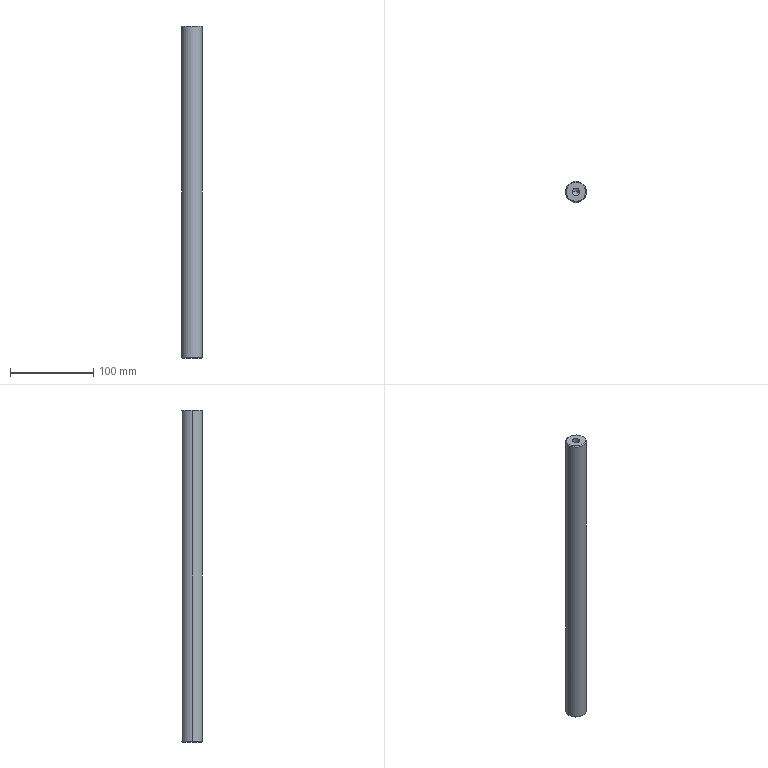Part | SolidWorks | features Chamfer 1, Extrusion 1, HoleWzd 1 | 1 solid | 12 faces | box 25 x 25 x 400 mm | volume 194835 mm3 | cone 6 | cylinder 4 | plane 2 | commonest cylinder face diameters 8.5 x2 25 x2
STEP:
#1=CARTESIAN_POINT('',(-4.25,0.,175.5));
#2=VERTEX_POINT('',#1);
#3=CARTESIAN_POINT('',(4.25,0.,175.5));
#4=VERTEX_POINT('',#3);
#5=CARTESIAN_POINT('',(0.,0.,175.5));
#6=DIRECTION('',(0.,0.,1.));
#7=DIRECTION('',(1.,0.,0.));
#8=AXIS2_PLACEMENT_3D('',#5,#6,#7);
#9=CIRCLE('',#8,4.25);
#10=EDGE_CURVE('',#2,#4,#9,.T.);
#11=ORIENTED_EDGE('',*,*,#10,.F.);
#12=CARTESIAN_POINT('',(-4.25,0.,200.));
#13=VERTEX_POINT('',#12);
#14=CARTESIAN_POINT('',(-4.25,0.,200.));
#15=DIRECTION('',(0.,0.,1.));
#16=VECTOR('',#15,1000.);
#17=LINE('',#14,#16);
#18=EDGE_CURVE('',#2,#13,#17,.T.);
#19=ORIENTED_EDGE('',*,*,#18,.T.);
#20=CARTESIAN_POINT('',(4.25,0.,200.));
#21=VERTEX_POINT('',#20);
#22=CARTESIAN_POINT('',(0.,0.,200.));
#23=DIRECTION('',(0.,0.,1.));
#24=DIRECTION('',(1.,0.,0.));
#25=AXIS2_PLACEMENT_3D('',#22,#23,#24);
#26=CIRCLE('',#25,4.25);
#27=EDGE_CURVE('',#13,#21,#26,.T.);
#28=ORIENTED_EDGE('',*,*,#27,.T.);
#29=CARTESIAN_POINT('',(4.25,0.,200.));
#30=DIRECTION('',(0.,0.,1.));
#31=VECTOR('',#30,1000.);
#32=LINE('',#29,#31);
#33=EDGE_CURVE('',#4,#21,#32,.T.);
#34=ORIENTED_EDGE('',*,*,#33,.F.);
#35=EDGE_LOOP('',(#11,#19,#28,#34));
#36=FACE_OUTER_BOUND('',#35,.T.);
#37=CARTESIAN_POINT('',(0.,0.,200.));
#38=DIRECTION('',(0.,0.,1.));
#39=DIRECTION('',(1.,0.,0.));
#40=AXIS2_PLACEMENT_3D('',#37,#38,#39);
#41=CYLINDRICAL_SURFACE('',#40,4.25);
#42=ADVANCED_FACE('',(#36),#41,.F.);
#43=CARTESIAN_POINT('',(0.,0.,172.946));
#44=VERTEX_POINT('',#43);
#45=CARTESIAN_POINT('',(4.25,0.,175.5));
#46=DIRECTION('',(0.8572,0.,0.515));
#47=VECTOR('',#46,1000.);
#48=LINE('',#45,#47);
#49=EDGE_CURVE('',#44,#4,#48,.T.);
#50=ORIENTED_EDGE('',*,*,#49,.F.);
#51=CARTESIAN_POINT('',(-4.25,0.,175.5));
#52=DIRECTION('',(-0.8572,0.,0.515));
#53=VECTOR('',#52,1000.);
#54=LINE('',#51,#53);
#55=EDGE_CURVE('',#44,#2,#54,.T.);
#56=ORIENTED_EDGE('',*,*,#55,.T.);
#57=ORIENTED_EDGE('',*,*,#10,.T.);
#58=EDGE_LOOP('',(#50,#56,#57));
#59=FACE_OUTER_BOUND('',#58,.T.);
#60=CARTESIAN_POINT('',(0.,0.,175.5));
#61=DIRECTION('',(0.,0.,1.));
#62=DIRECTION('',(1.,0.,0.));
#63=AXIS2_PLACEMENT_3D('',#60,#61,#62);
#64=CONICAL_SURFACE('',#63,4.25,1.03);
#65=ADVANCED_FACE('',(#59),#64,.F.);
#66=CARTESIAN_POINT('',(11.5,0.,200.));
#67=VERTEX_POINT('',#66);
#68=CARTESIAN_POINT('',(-11.5,0.,200.));
#69=VERTEX_POINT('',#68);
#70=CARTESIAN_POINT('',(0.,0.,200.));
#71=DIRECTION('',(0.,0.,1.));
#72=DIRECTION('',(1.,0.,0.));
#73=AXIS2_PLACEMENT_3D('',#70,#71,#72);
#74=CIRCLE('',#73,11.5);
#75=EDGE_CURVE('',#67,#69,#74,.T.);
#76=ORIENTED_EDGE('',*,*,#75,.F.);
#77=CARTESIAN_POINT('',(12.5,0.,199.));
#78=VERTEX_POINT('',#77);
#79=CARTESIAN_POINT('',(11.5,0.,200.));
#80=DIRECTION('',(0.7071,0.,-0.7071));
#81=VECTOR('',#80,1000.);
#82=LINE('',#79,#81);
#83=EDGE_CURVE('',#67,#78,#82,.T.);
#84=ORIENTED_EDGE('',*,*,#83,.T.);
#85=CARTESIAN_POINT('',(-12.5,0.,199.));
#86=VERTEX_POINT('',#85);
#87=CARTESIAN_POINT('',(0.,0.,199.));
#88=DIRECTION('',(0.,0.,-1.));
#89=DIRECTION('',(1.,0.,0.));
#90=AXIS2_PLACEMENT_3D('',#87,#88,#89);
#91=CIRCLE('',#90,12.5);
#92=EDGE_CURVE('',#86,#78,#91,.T.);
#93=ORIENTED_EDGE('',*,*,#92,.F.);
#94=CARTESIAN_POINT('',(-11.5,0.,200.));
#95=DIRECTION('',(-0.7071,0.,-0.7071));
#96=VECTOR('',#95,1000.);
#97=LINE('',#94,#96);
#98=EDGE_CURVE('',#69,#86,#97,.T.);
#99=ORIENTED_EDGE('',*,*,#98,.F.);
#100=EDGE_LOOP('',(#76,#84,#93,#99));
#101=FACE_OUTER_BOUND('',#100,.T.);
#102=CARTESIAN_POINT('',(0.,0.,200.));
#103=DIRECTION('',(0.,0.,-1.));
#104=DIRECTION('',(-1.,0.,0.));
#105=AXIS2_PLACEMENT_3D('',#102,#103,#104);
#106=CONICAL_SURFACE('',#105,11.5,0.7854);
#107=ADVANCED_FACE('',(#101),#106,.T.);
#108=CARTESIAN_POINT('',(-11.5,0.,-200.));
#109=VERTEX_POINT('',#108);
#110=CARTESIAN_POINT('',(11.5,0.,-200.));
#111=VERTEX_POINT('',#110);
#112=CARTESIAN_POINT('',(0.,0.,-200.));
#113=DIRECTION('',(0.,0.,-1.));
#114=DIRECTION('',(1.,0.,0.));
#115=AXIS2_PLACEMENT_3D('',#112,#113,#114);
#116=CIRCLE('',#115,11.5);
#117=EDGE_CURVE('',#109,#111,#116,.T.);
#118=ORIENTED_EDGE('',*,*,#117,.F.);
#119=CARTESIAN_POINT('',(-12.5,0.,-199.));
#120=VERTEX_POINT('',#119);
#121=CARTESIAN_POINT('',(-12.5,0.,-199.));
#122=DIRECTION('',(-0.7071,0.,0.7071));
#123=VECTOR('',#122,1000.);
#124=LINE('',#121,#123);
#125=EDGE_CURVE('',#109,#120,#124,.T.);
#126=ORIENTED_EDGE('',*,*,#125,.T.);
#127=CARTESIAN_POINT('',(12.5,0.,-199.));
#128=VERTEX_POINT('',#127);
#129=CARTESIAN_POINT('',(0.,0.,-199.));
#130=DIRECTION('',(0.,0.,1.));
#131=DIRECTION('',(1.,0.,0.));
#132=AXIS2_PLACEMENT_3D('',#129,#130,#131);
#133=CIRCLE('',#132,12.5);
#134=EDGE_CURVE('',#128,#120,#133,.T.);
#135=ORIENTED_EDGE('',*,*,#134,.F.);
#136=CARTESIAN_POINT('',(12.5,0.,-199.));
#137=DIRECTION('',(0.7071,0.,0.7071));
#138=VECTOR('',#137,1000.);
#139=LINE('',#136,#138);
#140=EDGE_CURVE('',#111,#128,#139,.T.);
#141=ORIENTED_EDGE('',*,*,#140,.F.);
#142=EDGE_LOOP('',(#118,#126,#135,#141));
#143=FACE_OUTER_BOUND('',#142,.T.);
#144=CARTESIAN_POINT('',(0.,0.,-199.));
#145=DIRECTION('',(0.,0.,1.));
#146=DIRECTION('',(1.,0.,0.));
#147=AXIS2_PLACEMENT_3D('',#144,#145,#146);
#148=CONICAL_SURFACE('',#147,12.5,0.7854);
#149=ADVANCED_FACE('',(#143),#148,.T.);
#150=ORIENTED_EDGE('',*,*,#92,.T.);
#151=CARTESIAN_POINT('',(12.5,0.,200.));
#152=DIRECTION('',(0.,0.,-1.));
#153=VECTOR('',#152,1000.);
#154=LINE('',#151,#153);
#155=EDGE_CURVE('',#78,#128,#154,.T.);
#156=ORIENTED_EDGE('',*,*,#155,.T.);
#157=ORIENTED_EDGE('',*,*,#134,.T.);
#158=CARTESIAN_POINT('',(-12.5,0.,200.));
#159=DIRECTION('',(0.,0.,-1.));
#160=VECTOR('',#159,1000.);
#161=LINE('',#158,#160);
#162=EDGE_CURVE('',#86,#120,#161,.T.);
#163=ORIENTED_EDGE('',*,*,#162,.F.);
#164=EDGE_LOOP('',(#150,#156,#157,#163));
#165=FACE_OUTER_BOUND('',#164,.T.);
#166=CARTESIAN_POINT('',(0.,0.,200.));
#167=DIRECTION('',(0.,0.,-1.));
#168=DIRECTION('',(-1.,0.,0.));
#169=AXIS2_PLACEMENT_3D('',#166,#167,#168);
#170=CYLINDRICAL_SURFACE('',#169,12.5);
#171=ADVANCED_FACE('',(#165),#170,.T.);
#172=ORIENTED_EDGE('',*,*,#155,.F.);
#173=CARTESIAN_POINT('',(0.,0.,199.));
#174=DIRECTION('',(0.,0.,-1.));
#175=DIRECTION('',(1.,0.,0.));
#176=AXIS2_PLACEMENT_3D('',#173,#174,#175);
#177=CIRCLE('',#176,12.5);
#178=EDGE_CURVE('',#78,#86,#177,.T.);
#179=ORIENTED_EDGE('',*,*,#178,.T.);
#180=ORIENTED_EDGE('',*,*,#162,.T.);
#181=CARTESIAN_POINT('',(0.,0.,-199.));
#182=DIRECTION('',(0.,0.,1.));
#183=DIRECTION('',(1.,0.,0.));
#184=AXIS2_PLACEMENT_3D('',#181,#182,#183);
#185=CIRCLE('',#184,12.5);
#186=EDGE_CURVE('',#120,#128,#185,.T.);
#187=ORIENTED_EDGE('',*,*,#186,.T.);
#188=EDGE_LOOP('',(#172,#179,#180,#187));
#189=FACE_OUTER_BOUND('',#188,.T.);
#190=CARTESIAN_POINT('',(0.,0.,200.));
#191=DIRECTION('',(0.,0.,-1.));
#192=DIRECTION('',(-1.,0.,0.));
#193=AXIS2_PLACEMENT_3D('',#190,#191,#192);
#194=CYLINDRICAL_SURFACE('',#193,12.5);
#195=ADVANCED_FACE('',(#189),#194,.T.);
#196=CARTESIAN_POINT('',(0.,0.,200.));
#197=DIRECTION('',(0.,0.,1.));
#198=DIRECTION('',(1.,0.,0.));
#199=AXIS2_PLACEMENT_3D('',#196,#197,#198);
#200=CIRCLE('',#199,4.25);
#201=EDGE_CURVE('',#21,#13,#200,.T.);
#202=ORIENTED_EDGE('',*,*,#201,.F.);
#203=ORIENTED_EDGE('',*,*,#27,.F.);
#204=EDGE_LOOP('',(#202,#203));
#205=FACE_BOUND('',#204,.T.);
#206=CARTESIAN_POINT('',(0.,0.,200.));
#207=DIRECTION('',(0.,0.,1.));
#208=DIRECTION('',(1.,0.,0.));
#209=AXIS2_PLACEMENT_3D('',#206,#207,#208);
#210=CIRCLE('',#209,11.5);
#211=EDGE_CURVE('',#69,#67,#210,.T.);
#212=ORIENTED_EDGE('',*,*,#211,.T.);
#213=ORIENTED_EDGE('',*,*,#75,.T.);
#214=EDGE_LOOP('',(#212,#213));
#215=FACE_OUTER_BOUND('',#214,.T.);
#216=CARTESIAN_POINT('',(0.,0.,200.));
#217=DIRECTION('',(0.,0.,1.));
#218=DIRECTION('',(1.,0.,0.));
#219=AXIS2_PLACEMENT_3D('',#216,#217,#218);
#220=PLANE('',#219);
#221=ADVANCED_FACE('',(#205,#215),#220,.T.);
#222=CARTESIAN_POINT('',(0.,0.,-200.));
#223=DIRECTION('',(0.,0.,-1.));
#224=DIRECTION('',(1.,0.,0.));
#225=AXIS2_PLACEMENT_3D('',#222,#223,#224);
#226=CIRCLE('',#225,11.5);
#227=EDGE_CURVE('',#111,#109,#226,.T.);
#228=ORIENTED_EDGE('',*,*,#227,.T.);
#229=ORIENTED_EDGE('',*,*,#117,.T.);
#230=EDGE_LOOP('',(#228,#229));
#231=FACE_OUTER_BOUND('',#230,.T.);
#232=CARTESIAN_POINT('',(0.,0.,-200.));
#233=DIRECTION('',(0.,0.,1.));
#234=DIRECTION('',(1.,0.,0.));
#235=AXIS2_PLACEMENT_3D('',#232,#233,#234);
#236=PLANE('',#235);
#237=ADVANCED_FACE('',(#231),#236,.F.);
#238=ORIENTED_EDGE('',*,*,#125,.F.);
#239=ORIENTED_EDGE('',*,*,#227,.F.);
#240=ORIENTED_EDGE('',*,*,#140,.T.);
#241=ORIENTED_EDGE('',*,*,#186,.F.);
#242=EDGE_LOOP('',(#238,#239,#240,#241));
#243=FACE_OUTER_BOUND('',#242,.T.);
#244=CARTESIAN_POINT('',(0.,0.,-199.));
#245=DIRECTION('',(0.,0.,1.));
#246=DIRECTION('',(1.,0.,0.));
#247=AXIS2_PLACEMENT_3D('',#244,#245,#246);
#248=CONICAL_SURFACE('',#247,12.5,0.7854);
#249=ADVANCED_FACE('',(#243),#248,.T.);
#250=ORIENTED_EDGE('',*,*,#83,.F.);
#251=ORIENTED_EDGE('',*,*,#211,.F.);
#252=ORIENTED_EDGE('',*,*,#98,.T.);
#253=ORIENTED_EDGE('',*,*,#178,.F.);
#254=EDGE_LOOP('',(#250,#251,#252,#253));
#255=FACE_OUTER_BOUND('',#254,.T.);
#256=CARTESIAN_POINT('',(0.,0.,200.));
#257=DIRECTION('',(0.,0.,-1.));
#258=DIRECTION('',(-1.,0.,0.));
#259=AXIS2_PLACEMENT_3D('',#256,#257,#258);
#260=CONICAL_SURFACE('',#259,11.5,0.7854);
#261=ADVANCED_FACE('',(#255),#260,.T.);
#262=ORIENTED_EDGE('',*,*,#55,.F.);
#263=ORIENTED_EDGE('',*,*,#49,.T.);
#264=CARTESIAN_POINT('',(0.,0.,175.5));
#265=DIRECTION('',(0.,0.,1.));
#266=DIRECTION('',(1.,0.,0.));
#267=AXIS2_PLACEMENT_3D('',#264,#265,#266);
#268=CIRCLE('',#267,4.25);
#269=EDGE_CURVE('',#4,#2,#268,.T.);
#270=ORIENTED_EDGE('',*,*,#269,.T.);
#271=EDGE_LOOP('',(#262,#263,#270));
#272=FACE_OUTER_BOUND('',#271,.T.);
#273=CARTESIAN_POINT('',(0.,0.,175.5));
#274=DIRECTION('',(0.,0.,1.));
#275=DIRECTION('',(1.,0.,0.));
#276=AXIS2_PLACEMENT_3D('',#273,#274,#275);
#277=CONICAL_SURFACE('',#276,4.25,1.03);
#278=ADVANCED_FACE('',(#272),#277,.F.);
#279=ORIENTED_EDGE('',*,*,#18,.F.);
#280=ORIENTED_EDGE('',*,*,#269,.F.);
#281=ORIENTED_EDGE('',*,*,#33,.T.);
#282=ORIENTED_EDGE('',*,*,#201,.T.);
#283=EDGE_LOOP('',(#279,#280,#281,#282));
#284=FACE_OUTER_BOUND('',#283,.T.);
#285=CARTESIAN_POINT('',(0.,0.,200.));
#286=DIRECTION('',(0.,0.,1.));
#287=DIRECTION('',(1.,0.,0.));
#288=AXIS2_PLACEMENT_3D('',#285,#286,#287);
#289=CYLINDRICAL_SURFACE('',#288,4.25);
#290=ADVANCED_FACE('',(#284),#289,.F.);
#291=CLOSED_SHELL('',(#42,#65,#107,#149,#171,#195,#221,#237,#249,#261,#278,#290));
#292=MANIFOLD_SOLID_BREP('',#291);
#293=CARTESIAN_POINT('',(0.,0.,0.));
#294=DIRECTION('',(0.,0.,1.));
#295=DIRECTION('',(1.,0.,0.));
#296=AXIS2_PLACEMENT_3D('',#293,#294,#295);
#297=(LENGTH_UNIT()NAMED_UNIT(*)SI_UNIT(.MILLI.,.METRE.));
#298=UNCERTAINTY_MEASURE_WITH_UNIT(LENGTH_MEASURE(0.00001),#297,'','');
#299=(NAMED_UNIT(*)PLANE_ANGLE_UNIT()SI_UNIT($,.RADIAN.));
#300=(NAMED_UNIT(*)SI_UNIT($,.STERADIAN.)SOLID_ANGLE_UNIT());
#301=(GEOMETRIC_REPRESENTATION_CONTEXT(3)GLOBAL_UNCERTAINTY_ASSIGNED_CONTEXT((#298))GLOBAL_UNIT_ASSIGNED_CONTEXT((#297,#299,#300))REPRESENTATION_CONTEXT('',''));
#302=ADVANCED_BREP_SHAPE_REPRESENTATION('',(#292,#296),#301);